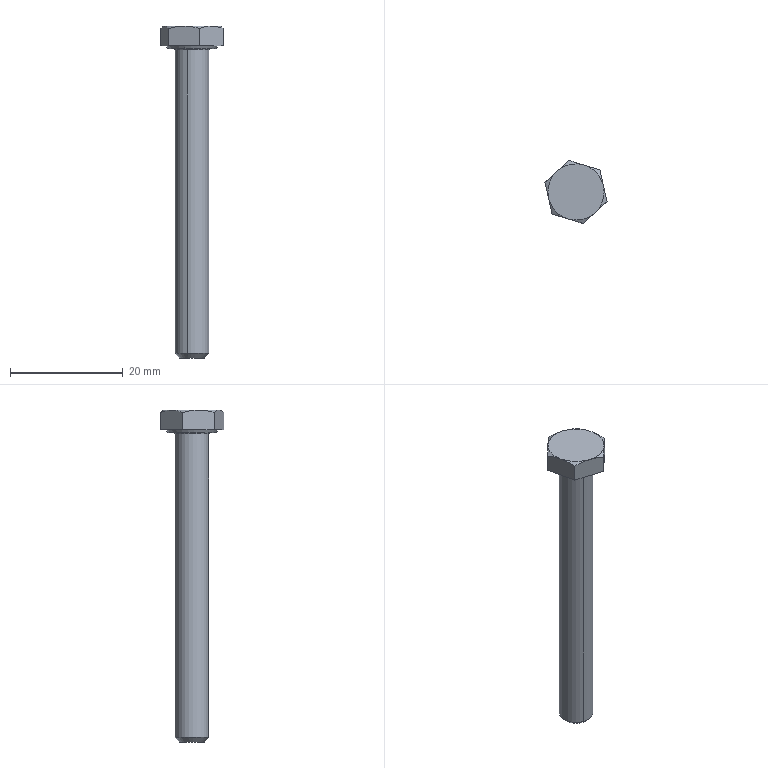Part | STEP file | BFACE2-18 | 1 solid | 24 faces | box 11.042 x 11.251 x 59 mm | volume 1883 mm3 | cone 10 | plane 10 | cylinder 2 | torus 2 | commonest cylinder face diameters 6 x2
STEP:
#1=CARTESIAN_POINT('',(-616.616,-367.304,3117.75));
#2=VERTEX_POINT('',#1);
#3=CARTESIAN_POINT('',(-614.861,-361.566,3117.75));
#4=VERTEX_POINT('',#3);
#5=CARTESIAN_POINT('',(-615.738,-364.435,3117.75));
#6=DIRECTION('',(0.,0.,1.));
#7=DIRECTION('',(-0.2924,-0.9563,0.));
#8=AXIS2_PLACEMENT_3D('',#5,#6,#7);
#9=CIRCLE('',#8,3.);
#10=EDGE_CURVE('',#2,#4,#9,.T.);
#11=ORIENTED_EDGE('',*,*,#10,.F.);
#12=CARTESIAN_POINT('',(-616.616,-367.304,3063.8));
#13=VERTEX_POINT('',#12);
#14=CARTESIAN_POINT('',(-616.616,-367.304,3122.));
#15=DIRECTION('',(0.,0.,1.));
#16=VECTOR('',#15,1000.);
#17=LINE('',#14,#16);
#18=EDGE_CURVE('',#13,#2,#17,.T.);
#19=ORIENTED_EDGE('',*,*,#18,.F.);
#20=CARTESIAN_POINT('',(-614.861,-361.566,3063.8));
#21=VERTEX_POINT('',#20);
#22=CARTESIAN_POINT('',(-615.738,-364.435,3063.8));
#23=DIRECTION('',(0.,0.,1.));
#24=DIRECTION('',(0.2924,0.9563,0.));
#25=AXIS2_PLACEMENT_3D('',#22,#23,#24);
#26=CIRCLE('',#25,3.);
#27=EDGE_CURVE('',#13,#21,#26,.T.);
#28=ORIENTED_EDGE('',*,*,#27,.T.);
#29=CARTESIAN_POINT('',(-614.861,-361.566,3122.));
#30=DIRECTION('',(0.,0.,1.));
#31=VECTOR('',#30,1000.);
#32=LINE('',#29,#31);
#33=EDGE_CURVE('',#21,#4,#32,.T.);
#34=ORIENTED_EDGE('',*,*,#33,.T.);
#35=EDGE_LOOP('',(#11,#19,#28,#34));
#36=FACE_OUTER_BOUND('',#35,.T.);
#37=CARTESIAN_POINT('',(-615.738,-364.435,3122.));
#38=DIRECTION('',(0.,0.,-1.));
#39=DIRECTION('',(-0.2924,-0.9563,0.));
#40=AXIS2_PLACEMENT_3D('',#37,#38,#39);
#41=CYLINDRICAL_SURFACE('',#40,3.);
#42=ADVANCED_FACE('',(#36),#41,.T.);
#43=CARTESIAN_POINT('',(-615.095,-362.331,3063.));
#44=VERTEX_POINT('',#43);
#45=CARTESIAN_POINT('',(-616.382,-366.539,3063.));
#46=VERTEX_POINT('',#45);
#47=CARTESIAN_POINT('',(-615.738,-364.435,3063.));
#48=DIRECTION('',(0.,0.,-1.));
#49=DIRECTION('',(0.2924,0.9563,0.));
#50=AXIS2_PLACEMENT_3D('',#47,#48,#49);
#51=CIRCLE('',#50,2.2);
#52=EDGE_CURVE('',#44,#46,#51,.T.);
#53=ORIENTED_EDGE('',*,*,#52,.F.);
#54=CARTESIAN_POINT('',(-615.095,-362.331,3063.));
#55=DIRECTION('',(0.2068,0.6762,0.7071));
#56=VECTOR('',#55,1000.);
#57=LINE('',#54,#56);
#58=EDGE_CURVE('',#44,#21,#57,.T.);
#59=ORIENTED_EDGE('',*,*,#58,.T.);
#60=ORIENTED_EDGE('',*,*,#27,.F.);
#61=CARTESIAN_POINT('',(-616.382,-366.539,3063.));
#62=DIRECTION('',(-0.2068,-0.6762,0.7071));
#63=VECTOR('',#62,1000.);
#64=LINE('',#61,#63);
#65=EDGE_CURVE('',#46,#13,#64,.T.);
#66=ORIENTED_EDGE('',*,*,#65,.F.);
#67=EDGE_LOOP('',(#53,#59,#60,#66));
#68=FACE_OUTER_BOUND('',#67,.T.);
#69=CARTESIAN_POINT('',(-615.738,-364.435,3063.));
#70=DIRECTION('',(0.,0.,1.));
#71=DIRECTION('',(0.2924,0.9563,0.));
#72=AXIS2_PLACEMENT_3D('',#69,#70,#71);
#73=CONICAL_SURFACE('',#72,2.2,0.7854);
#74=ADVANCED_FACE('',(#68),#73,.T.);
#75=CARTESIAN_POINT('',(-614.788,-361.327,3118.));
#76=VERTEX_POINT('',#75);
#77=CARTESIAN_POINT('',(-616.689,-367.543,3118.));
#78=VERTEX_POINT('',#77);
#79=CARTESIAN_POINT('',(-615.738,-364.435,3118.));
#80=DIRECTION('',(0.,0.,1.));
#81=DIRECTION('',(-0.2924,-0.9563,0.));
#82=AXIS2_PLACEMENT_3D('',#79,#80,#81);
#83=CIRCLE('',#82,3.25);
#84=EDGE_CURVE('',#76,#78,#83,.T.);
#85=ORIENTED_EDGE('',*,*,#84,.F.);
#86=CARTESIAN_POINT('',(-614.788,-361.327,3117.75));
#87=DIRECTION('',(0.9563,-0.2924,0.));
#88=DIRECTION('',(-0.2924,-0.9563,0.));
#89=AXIS2_PLACEMENT_3D('',#86,#87,#88);
#90=CIRCLE('',#89,0.25);
#91=EDGE_CURVE('',#76,#4,#90,.T.);
#92=ORIENTED_EDGE('',*,*,#91,.T.);
#93=CARTESIAN_POINT('',(-615.738,-364.435,3117.75));
#94=DIRECTION('',(0.,0.,1.));
#95=DIRECTION('',(-0.2924,-0.9563,0.));
#96=AXIS2_PLACEMENT_3D('',#93,#94,#95);
#97=CIRCLE('',#96,3.);
#98=EDGE_CURVE('',#4,#2,#97,.T.);
#99=ORIENTED_EDGE('',*,*,#98,.T.);
#100=CARTESIAN_POINT('',(-616.689,-367.543,3117.75));
#101=DIRECTION('',(-0.9563,0.2924,0.));
#102=DIRECTION('',(0.2924,0.9563,0.));
#103=AXIS2_PLACEMENT_3D('',#100,#101,#102);
#104=CIRCLE('',#103,0.25);
#105=EDGE_CURVE('',#78,#2,#104,.T.);
#106=ORIENTED_EDGE('',*,*,#105,.F.);
#107=EDGE_LOOP('',(#85,#92,#99,#106));
#108=FACE_OUTER_BOUND('',#107,.T.);
#109=CARTESIAN_POINT('',(-615.738,-364.435,3117.75));
#110=DIRECTION('',(0.,0.,1.));
#111=DIRECTION('',(0.2924,0.9563,0.));
#112=AXIS2_PLACEMENT_3D('',#109,#110,#111);
#113=TOROIDAL_SURFACE('',#112,3.25,0.25);
#114=ADVANCED_FACE('',(#108),#113,.F.);
#115=CARTESIAN_POINT('',(-616.999,-368.559,3118.));
#116=VERTEX_POINT('',#115);
#117=CARTESIAN_POINT('',(-614.477,-360.311,3118.));
#118=VERTEX_POINT('',#117);
#119=CARTESIAN_POINT('',(-615.738,-364.435,3118.));
#120=DIRECTION('',(0.,0.,1.));
#121=DIRECTION('',(-0.2924,-0.9563,0.));
#122=AXIS2_PLACEMENT_3D('',#119,#120,#121);
#123=CIRCLE('',#122,4.312);
#124=EDGE_CURVE('',#116,#118,#123,.T.);
#125=ORIENTED_EDGE('',*,*,#124,.T.);
#126=CARTESIAN_POINT('',(-614.393,-360.035,3118.5));
#127=VERTEX_POINT('',#126);
#128=CARTESIAN_POINT('',(-614.393,-360.035,3118.5));
#129=DIRECTION('',(0.1462,0.4781,0.866));
#130=VECTOR('',#129,1000.);
#131=LINE('',#128,#130);
#132=EDGE_CURVE('',#118,#127,#131,.T.);
#133=ORIENTED_EDGE('',*,*,#132,.T.);
#134=CARTESIAN_POINT('',(-617.084,-368.835,3118.5));
#135=VERTEX_POINT('',#134);
#136=CARTESIAN_POINT('',(-615.738,-364.435,3118.5));
#137=DIRECTION('',(0.,0.,1.));
#138=DIRECTION('',(-0.2924,-0.9563,0.));
#139=AXIS2_PLACEMENT_3D('',#136,#137,#138);
#140=CIRCLE('',#139,4.601);
#141=EDGE_CURVE('',#135,#127,#140,.T.);
#142=ORIENTED_EDGE('',*,*,#141,.F.);
#143=CARTESIAN_POINT('',(-617.084,-368.835,3118.5));
#144=DIRECTION('',(-0.1462,-0.4781,0.866));
#145=VECTOR('',#144,1000.);
#146=LINE('',#143,#145);
#147=EDGE_CURVE('',#116,#135,#146,.T.);
#148=ORIENTED_EDGE('',*,*,#147,.F.);
#149=EDGE_LOOP('',(#125,#133,#142,#148));
#150=FACE_OUTER_BOUND('',#149,.T.);
#151=CARTESIAN_POINT('',(-615.738,-364.435,3118.5));
#152=DIRECTION('',(0.,0.,1.));
#153=DIRECTION('',(0.2924,0.9563,0.));
#154=AXIS2_PLACEMENT_3D('',#151,#152,#153);
#155=CONICAL_SURFACE('',#154,4.601,0.5236);
#156=ADVANCED_FACE('',(#150),#155,.T.);
#157=ORIENTED_EDGE('',*,*,#124,.F.);
#158=CARTESIAN_POINT('',(-615.738,-364.435,3118.));
#159=DIRECTION('',(0.,0.,1.));
#160=DIRECTION('',(-0.2924,-0.9563,0.));
#161=AXIS2_PLACEMENT_3D('',#158,#159,#160);
#162=CIRCLE('',#161,4.312);
#163=EDGE_CURVE('',#118,#116,#162,.T.);
#164=ORIENTED_EDGE('',*,*,#163,.F.);
#165=EDGE_LOOP('',(#157,#164));
#166=FACE_OUTER_BOUND('',#165,.T.);
#167=CARTESIAN_POINT('',(-615.738,-364.435,3118.));
#168=DIRECTION('',(0.,0.,1.));
#169=DIRECTION('',(-0.2924,-0.9563,0.));
#170=AXIS2_PLACEMENT_3D('',#167,#168,#169);
#171=CIRCLE('',#170,3.25);
#172=EDGE_CURVE('',#78,#76,#171,.T.);
#173=ORIENTED_EDGE('',*,*,#172,.T.);
#174=ORIENTED_EDGE('',*,*,#84,.T.);
#175=EDGE_LOOP('',(#173,#174));
#176=FACE_BOUND('',#175,.T.);
#177=CARTESIAN_POINT('',(-610.217,-366.123,3118.));
#178=DIRECTION('',(0.,0.,-1.));
#179=DIRECTION('',(-0.2924,-0.9563,0.));
#180=AXIS2_PLACEMENT_3D('',#177,#178,#179);
#181=PLANE('',#180);
#182=ADVANCED_FACE('',(#166,#176),#181,.T.);
#183=CARTESIAN_POINT('',(-611.516,-360.498,3118.5));
#184=VERTEX_POINT('',#183);
#185=CARTESIAN_POINT('',(-610.217,-366.123,3118.5));
#186=VERTEX_POINT('',#185);
#187=CARTESIAN_POINT('',(-611.516,-360.498,3118.5));
#188=DIRECTION('',(0.2249,-0.9744,0.));
#189=VECTOR('',#188,1000.);
#190=LINE('',#187,#189);
#191=EDGE_CURVE('',#184,#186,#190,.T.);
#192=ORIENTED_EDGE('',*,*,#191,.F.);
#193=CARTESIAN_POINT('',(-611.516,-360.498,3121.553));
#194=VERTEX_POINT('',#193);
#195=CARTESIAN_POINT('',(-611.516,-360.498,3118.));
#196=DIRECTION('',(0.,0.,1.));
#197=VECTOR('',#196,1000.);
#198=LINE('',#195,#197);
#199=EDGE_CURVE('',#184,#194,#198,.T.);
#200=ORIENTED_EDGE('',*,*,#199,.T.);
#201=CARTESIAN_POINT('',(-610.866,-363.311,3122.));
#202=VERTEX_POINT('',#201);
#203=CARTESIAN_POINT('',(-610.866,-363.311,3122.));
#204=CARTESIAN_POINT('',(-611.088,-362.351,3122.));
#205=CARTESIAN_POINT('',(-611.303,-361.417,3121.826));
#206=CARTESIAN_POINT('',(-611.516,-360.498,3121.553));
#207=B_SPLINE_CURVE_WITH_KNOTS('',3,(#203,#204,#205,#206),.UNSPECIFIED.,.F.,.F.,(4,4),(0.,0.002921),.UNSPECIFIED.);
#208=EDGE_CURVE('',#202,#194,#207,.T.);
#209=ORIENTED_EDGE('',*,*,#208,.F.);
#210=CARTESIAN_POINT('',(-610.217,-366.123,3121.553));
#211=VERTEX_POINT('',#210);
#212=CARTESIAN_POINT('',(-610.217,-366.123,3121.553));
#213=CARTESIAN_POINT('',(-610.429,-365.204,3121.826));
#214=CARTESIAN_POINT('',(-610.645,-364.271,3122.));
#215=CARTESIAN_POINT('',(-610.866,-363.311,3122.));
#216=B_SPLINE_CURVE_WITH_KNOTS('',3,(#212,#213,#214,#215),.UNSPECIFIED.,.F.,.F.,(4,4),(0.,0.002921),.UNSPECIFIED.);
#217=EDGE_CURVE('',#211,#202,#216,.T.);
#218=ORIENTED_EDGE('',*,*,#217,.F.);
#219=CARTESIAN_POINT('',(-610.217,-366.123,3118.));
#220=DIRECTION('',(0.,0.,1.));
#221=VECTOR('',#220,1000.);
#222=LINE('',#219,#221);
#223=EDGE_CURVE('',#186,#211,#222,.T.);
#224=ORIENTED_EDGE('',*,*,#223,.F.);
#225=EDGE_LOOP('',(#192,#200,#209,#218,#224));
#226=FACE_OUTER_BOUND('',#225,.T.);
#227=CARTESIAN_POINT('',(-611.516,-360.498,3118.));
#228=DIRECTION('',(-0.9744,-0.2249,0.));
#229=DIRECTION('',(0.2249,-0.9744,0.));
#230=AXIS2_PLACEMENT_3D('',#227,#228,#229);
#231=PLANE('',#230);
#232=ADVANCED_FACE('',(#226),#231,.F.);
#233=CARTESIAN_POINT('',(-614.44,-370.061,3118.5));
#234=VERTEX_POINT('',#233);
#235=CARTESIAN_POINT('',(-610.217,-366.123,3118.5));
#236=DIRECTION('',(-0.7314,-0.682,0.));
#237=VECTOR('',#236,1000.);
#238=LINE('',#235,#237);
#239=EDGE_CURVE('',#186,#234,#238,.T.);
#240=ORIENTED_EDGE('',*,*,#239,.F.);
#241=ORIENTED_EDGE('',*,*,#223,.T.);
#242=CARTESIAN_POINT('',(-612.329,-368.092,3122.));
#243=VERTEX_POINT('',#242);
#244=CARTESIAN_POINT('',(-612.329,-368.092,3122.));
#245=CARTESIAN_POINT('',(-611.608,-367.42,3122.));
#246=CARTESIAN_POINT('',(-610.907,-366.767,3121.826));
#247=CARTESIAN_POINT('',(-610.217,-366.123,3121.553));
#248=B_SPLINE_CURVE_WITH_KNOTS('',3,(#244,#245,#246,#247),.UNSPECIFIED.,.F.,.F.,(4,4),(0.,0.002921),.UNSPECIFIED.);
#249=EDGE_CURVE('',#243,#211,#248,.T.);
#250=ORIENTED_EDGE('',*,*,#249,.F.);
#251=CARTESIAN_POINT('',(-614.44,-370.061,3121.553));
#252=VERTEX_POINT('',#251);
#253=CARTESIAN_POINT('',(-614.44,-370.061,3121.553));
#254=CARTESIAN_POINT('',(-613.75,-369.418,3121.826));
#255=CARTESIAN_POINT('',(-613.049,-368.764,3122.));
#256=CARTESIAN_POINT('',(-612.329,-368.092,3122.));
#257=B_SPLINE_CURVE_WITH_KNOTS('',3,(#253,#254,#255,#256),.UNSPECIFIED.,.F.,.F.,(4,4),(0.,0.002921),.UNSPECIFIED.);
#258=EDGE_CURVE('',#252,#243,#257,.T.);
#259=ORIENTED_EDGE('',*,*,#258,.F.);
#260=CARTESIAN_POINT('',(-614.44,-370.061,3118.));
#261=DIRECTION('',(0.,0.,1.));
#262=VECTOR('',#261,1000.);
#263=LINE('',#260,#262);
#264=EDGE_CURVE('',#234,#252,#263,.T.);
#265=ORIENTED_EDGE('',*,*,#264,.F.);
#266=EDGE_LOOP('',(#240,#241,#250,#259,#265));
#267=FACE_OUTER_BOUND('',#266,.T.);
#268=CARTESIAN_POINT('',(-610.217,-366.123,3118.));
#269=DIRECTION('',(-0.682,0.7314,0.));
#270=DIRECTION('',(-0.7314,-0.682,0.));
#271=AXIS2_PLACEMENT_3D('',#268,#269,#270);
#272=PLANE('',#271);
#273=ADVANCED_FACE('',(#267),#272,.F.);
#274=CARTESIAN_POINT('',(-619.961,-368.372,3118.5));
#275=VERTEX_POINT('',#274);
#276=CARTESIAN_POINT('',(-614.44,-370.061,3118.5));
#277=DIRECTION('',(-0.9563,0.2924,0.));
#278=VECTOR('',#277,1000.);
#279=LINE('',#276,#278);
#280=EDGE_CURVE('',#234,#275,#279,.T.);
#281=ORIENTED_EDGE('',*,*,#280,.F.);
#282=ORIENTED_EDGE('',*,*,#264,.T.);
#283=CARTESIAN_POINT('',(-617.2,-369.217,3122.));
#284=VERTEX_POINT('',#283);
#285=CARTESIAN_POINT('',(-617.2,-369.217,3122.));
#286=CARTESIAN_POINT('',(-616.258,-369.505,3122.));
#287=CARTESIAN_POINT('',(-615.342,-369.785,3121.826));
#288=CARTESIAN_POINT('',(-614.44,-370.061,3121.553));
#289=B_SPLINE_CURVE_WITH_KNOTS('',3,(#285,#286,#287,#288),.UNSPECIFIED.,.F.,.F.,(4,4),(0.,0.002921),.UNSPECIFIED.);
#290=EDGE_CURVE('',#284,#252,#289,.T.);
#291=ORIENTED_EDGE('',*,*,#290,.F.);
#292=CARTESIAN_POINT('',(-619.961,-368.372,3121.553));
#293=VERTEX_POINT('',#292);
#294=CARTESIAN_POINT('',(-619.961,-368.372,3121.553));
#295=CARTESIAN_POINT('',(-619.059,-368.648,3121.826));
#296=CARTESIAN_POINT('',(-618.143,-368.928,3122.));
#297=CARTESIAN_POINT('',(-617.2,-369.217,3122.));
#298=B_SPLINE_CURVE_WITH_KNOTS('',3,(#294,#295,#296,#297),.UNSPECIFIED.,.F.,.F.,(4,4),(0.,0.002921),.UNSPECIFIED.);
#299=EDGE_CURVE('',#293,#284,#298,.T.);
#300=ORIENTED_EDGE('',*,*,#299,.F.);
#301=CARTESIAN_POINT('',(-619.961,-368.372,3118.));
#302=DIRECTION('',(0.,0.,1.));
#303=VECTOR('',#302,1000.);
#304=LINE('',#301,#303);
#305=EDGE_CURVE('',#275,#293,#304,.T.);
#306=ORIENTED_EDGE('',*,*,#305,.F.);
#307=EDGE_LOOP('',(#281,#282,#291,#300,#306));
#308=FACE_OUTER_BOUND('',#307,.T.);
#309=CARTESIAN_POINT('',(-614.44,-370.061,3118.));
#310=DIRECTION('',(0.2924,0.9563,0.));
#311=DIRECTION('',(0.,0.,-1.));
#312=AXIS2_PLACEMENT_3D('',#309,#310,#311);
#313=PLANE('',#312);
#314=ADVANCED_FACE('',(#308),#313,.F.);
#315=CARTESIAN_POINT('',(-621.259,-362.747,3118.5));
#316=VERTEX_POINT('',#315);
#317=CARTESIAN_POINT('',(-621.259,-362.747,3118.5));
#318=DIRECTION('',(-0.2249,0.9744,0.));
#319=VECTOR('',#318,1000.);
#320=LINE('',#317,#319);
#321=EDGE_CURVE('',#275,#316,#320,.T.);
#322=ORIENTED_EDGE('',*,*,#321,.F.);
#323=ORIENTED_EDGE('',*,*,#305,.T.);
#324=CARTESIAN_POINT('',(-620.61,-365.56,3122.));
#325=VERTEX_POINT('',#324);
#326=CARTESIAN_POINT('',(-620.61,-365.56,3122.));
#327=CARTESIAN_POINT('',(-620.389,-366.52,3122.));
#328=CARTESIAN_POINT('',(-620.173,-367.453,3121.826));
#329=CARTESIAN_POINT('',(-619.961,-368.372,3121.553));
#330=B_SPLINE_CURVE_WITH_KNOTS('',3,(#326,#327,#328,#329),.UNSPECIFIED.,.F.,.F.,(4,4),(0.,0.002921),.UNSPECIFIED.);
#331=EDGE_CURVE('',#325,#293,#330,.T.);
#332=ORIENTED_EDGE('',*,*,#331,.F.);
#333=CARTESIAN_POINT('',(-621.259,-362.747,3121.553));
#334=VERTEX_POINT('',#333);
#335=CARTESIAN_POINT('',(-621.259,-362.747,3121.553));
#336=CARTESIAN_POINT('',(-621.047,-363.666,3121.826));
#337=CARTESIAN_POINT('',(-620.832,-364.6,3122.));
#338=CARTESIAN_POINT('',(-620.61,-365.56,3122.));
#339=B_SPLINE_CURVE_WITH_KNOTS('',3,(#335,#336,#337,#338),.UNSPECIFIED.,.F.,.F.,(4,4),(0.,0.002921),.UNSPECIFIED.);
#340=EDGE_CURVE('',#334,#325,#339,.T.);
#341=ORIENTED_EDGE('',*,*,#340,.F.);
#342=CARTESIAN_POINT('',(-621.259,-362.747,3118.));
#343=DIRECTION('',(0.,0.,1.));
#344=VECTOR('',#343,1000.);
#345=LINE('',#342,#344);
#346=EDGE_CURVE('',#316,#334,#345,.T.);
#347=ORIENTED_EDGE('',*,*,#346,.F.);
#348=EDGE_LOOP('',(#322,#323,#332,#341,#347));
#349=FACE_OUTER_BOUND('',#348,.T.);
#350=CARTESIAN_POINT('',(-621.259,-362.747,3118.));
#351=DIRECTION('',(0.9744,0.2249,0.));
#352=DIRECTION('',(-0.2249,0.9744,0.));
#353=AXIS2_PLACEMENT_3D('',#350,#351,#352);
#354=PLANE('',#353);
#355=ADVANCED_FACE('',(#349),#354,.F.);
#356=CARTESIAN_POINT('',(-617.037,-358.81,3118.5));
#357=VERTEX_POINT('',#356);
#358=CARTESIAN_POINT('',(-617.037,-358.81,3118.5));
#359=DIRECTION('',(0.7314,0.682,0.));
#360=VECTOR('',#359,1000.);
#361=LINE('',#358,#360);
#362=EDGE_CURVE('',#316,#357,#361,.T.);
#363=ORIENTED_EDGE('',*,*,#362,.F.);
#364=ORIENTED_EDGE('',*,*,#346,.T.);
#365=CARTESIAN_POINT('',(-619.148,-360.778,3122.));
#366=VERTEX_POINT('',#365);
#367=CARTESIAN_POINT('',(-619.148,-360.778,3122.));
#368=CARTESIAN_POINT('',(-619.869,-361.45,3122.));
#369=CARTESIAN_POINT('',(-620.57,-362.104,3121.826));
#370=CARTESIAN_POINT('',(-621.259,-362.747,3121.553));
#371=B_SPLINE_CURVE_WITH_KNOTS('',3,(#367,#368,#369,#370),.UNSPECIFIED.,.F.,.F.,(4,4),(0.,0.002921),.UNSPECIFIED.);
#372=EDGE_CURVE('',#366,#334,#371,.T.);
#373=ORIENTED_EDGE('',*,*,#372,.F.);
#374=CARTESIAN_POINT('',(-617.037,-358.81,3121.553));
#375=VERTEX_POINT('',#374);
#376=CARTESIAN_POINT('',(-617.037,-358.81,3121.553));
#377=CARTESIAN_POINT('',(-617.726,-359.453,3121.826));
#378=CARTESIAN_POINT('',(-618.427,-360.106,3122.));
#379=CARTESIAN_POINT('',(-619.148,-360.778,3122.));
#380=B_SPLINE_CURVE_WITH_KNOTS('',3,(#376,#377,#378,#379),.UNSPECIFIED.,.F.,.F.,(4,4),(0.,0.002921),.UNSPECIFIED.);
#381=EDGE_CURVE('',#375,#366,#380,.T.);
#382=ORIENTED_EDGE('',*,*,#381,.F.);
#383=CARTESIAN_POINT('',(-617.037,-358.81,3118.));
#384=DIRECTION('',(0.,0.,1.));
#385=VECTOR('',#384,1000.);
#386=LINE('',#383,#385);
#387=EDGE_CURVE('',#357,#375,#386,.T.);
#388=ORIENTED_EDGE('',*,*,#387,.F.);
#389=EDGE_LOOP('',(#363,#364,#373,#382,#388));
#390=FACE_OUTER_BOUND('',#389,.T.);
#391=CARTESIAN_POINT('',(-617.037,-358.81,3118.));
#392=DIRECTION('',(0.682,-0.7314,0.));
#393=DIRECTION('',(0.7314,0.682,0.));
#394=AXIS2_PLACEMENT_3D('',#391,#392,#393);
#395=PLANE('',#394);
#396=ADVANCED_FACE('',(#390),#395,.F.);
#397=CARTESIAN_POINT('',(-611.516,-360.498,3118.5));
#398=DIRECTION('',(0.9563,-0.2924,0.));
#399=VECTOR('',#398,1000.);
#400=LINE('',#397,#399);
#401=EDGE_CURVE('',#357,#184,#400,.T.);
#402=ORIENTED_EDGE('',*,*,#401,.F.);
#403=ORIENTED_EDGE('',*,*,#387,.T.);
#404=CARTESIAN_POINT('',(-614.276,-359.654,3122.));
#405=VERTEX_POINT('',#404);
#406=CARTESIAN_POINT('',(-614.276,-359.654,3122.));
#407=CARTESIAN_POINT('',(-615.218,-359.366,3122.));
#408=CARTESIAN_POINT('',(-616.135,-359.085,3121.826));
#409=CARTESIAN_POINT('',(-617.037,-358.81,3121.553));
#410=B_SPLINE_CURVE_WITH_KNOTS('',3,(#406,#407,#408,#409),.UNSPECIFIED.,.F.,.F.,(4,4),(0.,0.002921),.UNSPECIFIED.);
#411=EDGE_CURVE('',#405,#375,#410,.T.);
#412=ORIENTED_EDGE('',*,*,#411,.F.);
#413=CARTESIAN_POINT('',(-611.516,-360.498,3121.553));
#414=CARTESIAN_POINT('',(-612.417,-360.222,3121.826));
#415=CARTESIAN_POINT('',(-613.334,-359.942,3122.));
#416=CARTESIAN_POINT('',(-614.276,-359.654,3122.));
#417=B_SPLINE_CURVE_WITH_KNOTS('',3,(#413,#414,#415,#416),.UNSPECIFIED.,.F.,.F.,(4,4),(0.,0.002921),.UNSPECIFIED.);
#418=EDGE_CURVE('',#194,#405,#417,.T.);
#419=ORIENTED_EDGE('',*,*,#418,.F.);
#420=ORIENTED_EDGE('',*,*,#199,.F.);
#421=EDGE_LOOP('',(#402,#403,#412,#419,#420));
#422=FACE_OUTER_BOUND('',#421,.T.);
#423=CARTESIAN_POINT('',(-611.516,-360.498,3118.));
#424=DIRECTION('',(-0.2924,-0.9563,0.));
#425=DIRECTION('',(0.9563,-0.2924,0.));
#426=AXIS2_PLACEMENT_3D('',#423,#424,#425);
#427=PLANE('',#426);
#428=ADVANCED_FACE('',(#422),#427,.F.);
#429=ORIENTED_EDGE('',*,*,#381,.T.);
#430=CARTESIAN_POINT('',(-615.738,-364.435,3122.));
#431=DIRECTION('',(0.,0.,-1.));
#432=DIRECTION('',(0.2924,0.9563,0.));
#433=AXIS2_PLACEMENT_3D('',#430,#431,#432);
#434=CIRCLE('',#433,5.);
#435=EDGE_CURVE('',#366,#405,#434,.T.);
#436=ORIENTED_EDGE('',*,*,#435,.T.);
#437=ORIENTED_EDGE('',*,*,#411,.T.);
#438=EDGE_LOOP('',(#429,#436,#437));
#439=FACE_OUTER_BOUND('',#438,.T.);
#440=CARTESIAN_POINT('',(-615.738,-364.435,3122.));
#441=DIRECTION('',(0.,0.,-1.));
#442=DIRECTION('',(-0.2924,-0.9563,0.));
#443=AXIS2_PLACEMENT_3D('',#440,#441,#442);
#444=CONICAL_SURFACE('',#443,5.,1.047);
#445=ADVANCED_FACE('',(#439),#444,.T.);
#446=ORIENTED_EDGE('',*,*,#340,.T.);
#447=CARTESIAN_POINT('',(-615.738,-364.435,3122.));
#448=DIRECTION('',(0.,0.,-1.));
#449=DIRECTION('',(0.2924,0.9563,0.));
#450=AXIS2_PLACEMENT_3D('',#447,#448,#449);
#451=CIRCLE('',#450,5.);
#452=EDGE_CURVE('',#325,#366,#451,.T.);
#453=ORIENTED_EDGE('',*,*,#452,.T.);
#454=ORIENTED_EDGE('',*,*,#372,.T.);
#455=EDGE_LOOP('',(#446,#453,#454));
#456=FACE_OUTER_BOUND('',#455,.T.);
#457=CARTESIAN_POINT('',(-615.738,-364.435,3122.));
#458=DIRECTION('',(0.,0.,-1.));
#459=DIRECTION('',(-0.2924,-0.9563,0.));
#460=AXIS2_PLACEMENT_3D('',#457,#458,#459);
#461=CONICAL_SURFACE('',#460,5.,1.047);
#462=ADVANCED_FACE('',(#456),#461,.T.);
#463=ORIENTED_EDGE('',*,*,#299,.T.);
#464=CARTESIAN_POINT('',(-615.738,-364.435,3122.));
#465=DIRECTION('',(0.,0.,-1.));
#466=DIRECTION('',(0.2924,0.9563,0.));
#467=AXIS2_PLACEMENT_3D('',#464,#465,#466);
#468=CIRCLE('',#467,5.);
#469=EDGE_CURVE('',#284,#325,#468,.T.);
#470=ORIENTED_EDGE('',*,*,#469,.T.);
#471=ORIENTED_EDGE('',*,*,#331,.T.);
#472=EDGE_LOOP('',(#463,#470,#471));
#473=FACE_OUTER_BOUND('',#472,.T.);
#474=CARTESIAN_POINT('',(-615.738,-364.435,3122.));
#475=DIRECTION('',(0.,0.,-1.));
#476=DIRECTION('',(-0.2924,-0.9563,0.));
#477=AXIS2_PLACEMENT_3D('',#474,#475,#476);
#478=CONICAL_SURFACE('',#477,5.,1.047);
#479=ADVANCED_FACE('',(#473),#478,.T.);
#480=ORIENTED_EDGE('',*,*,#290,.T.);
#481=ORIENTED_EDGE('',*,*,#258,.T.);
#482=CARTESIAN_POINT('',(-615.738,-364.435,3122.));
#483=DIRECTION('',(0.,0.,1.));
#484=DIRECTION('',(-0.2924,-0.9563,0.));
#485=AXIS2_PLACEMENT_3D('',#482,#483,#484);
#486=CIRCLE('',#485,5.);
#487=EDGE_CURVE('',#284,#243,#486,.T.);
#488=ORIENTED_EDGE('',*,*,#487,.F.);
#489=EDGE_LOOP('',(#480,#481,#488));
#490=FACE_OUTER_BOUND('',#489,.T.);
#491=CARTESIAN_POINT('',(-615.738,-364.435,3122.));
#492=DIRECTION('',(0.,0.,-1.));
#493=DIRECTION('',(-0.2924,-0.9563,0.));
#494=AXIS2_PLACEMENT_3D('',#491,#492,#493);
#495=CONICAL_SURFACE('',#494,5.,1.047);
#496=ADVANCED_FACE('',(#490),#495,.T.);
#497=ORIENTED_EDGE('',*,*,#249,.T.);
#498=ORIENTED_EDGE('',*,*,#217,.T.);
#499=CARTESIAN_POINT('',(-615.738,-364.435,3122.));
#500=DIRECTION('',(0.,0.,-1.));
#501=DIRECTION('',(0.2924,0.9563,0.));
#502=AXIS2_PLACEMENT_3D('',#499,#500,#501);
#503=CIRCLE('',#502,5.);
#504=EDGE_CURVE('',#202,#243,#503,.T.);
#505=ORIENTED_EDGE('',*,*,#504,.T.);
#506=EDGE_LOOP('',(#497,#498,#505));
#507=FACE_OUTER_BOUND('',#506,.T.);
#508=CARTESIAN_POINT('',(-615.738,-364.435,3122.));
#509=DIRECTION('',(0.,0.,-1.));
#510=DIRECTION('',(-0.2924,-0.9563,0.));
#511=AXIS2_PLACEMENT_3D('',#508,#509,#510);
#512=CONICAL_SURFACE('',#511,5.,1.047);
#513=ADVANCED_FACE('',(#507),#512,.T.);
#514=ORIENTED_EDGE('',*,*,#208,.T.);
#515=ORIENTED_EDGE('',*,*,#418,.T.);
#516=CARTESIAN_POINT('',(-615.738,-364.435,3122.));
#517=DIRECTION('',(0.,0.,-1.));
#518=DIRECTION('',(0.2924,0.9563,0.));
#519=AXIS2_PLACEMENT_3D('',#516,#517,#518);
#520=CIRCLE('',#519,5.);
#521=EDGE_CURVE('',#405,#202,#520,.T.);
#522=ORIENTED_EDGE('',*,*,#521,.T.);
#523=EDGE_LOOP('',(#514,#515,#522));
#524=FACE_OUTER_BOUND('',#523,.T.);
#525=CARTESIAN_POINT('',(-615.738,-364.435,3122.));
#526=DIRECTION('',(0.,0.,-1.));
#527=DIRECTION('',(-0.2924,-0.9563,0.));
#528=AXIS2_PLACEMENT_3D('',#525,#526,#527);
#529=CONICAL_SURFACE('',#528,5.,1.047);
#530=ADVANCED_FACE('',(#524),#529,.T.);
#531=ORIENTED_EDGE('',*,*,#521,.F.);
#532=ORIENTED_EDGE('',*,*,#435,.F.);
#533=ORIENTED_EDGE('',*,*,#452,.F.);
#534=ORIENTED_EDGE('',*,*,#469,.F.);
#535=ORIENTED_EDGE('',*,*,#487,.T.);
#536=ORIENTED_EDGE('',*,*,#504,.F.);
#537=EDGE_LOOP('',(#531,#532,#533,#534,#535,#536));
#538=FACE_OUTER_BOUND('',#537,.T.);
#539=CARTESIAN_POINT('',(-610.217,-366.123,3122.));
#540=DIRECTION('',(0.,0.,-1.));
#541=DIRECTION('',(-0.2924,-0.9563,0.));
#542=AXIS2_PLACEMENT_3D('',#539,#540,#541);
#543=PLANE('',#542);
#544=ADVANCED_FACE('',(#538),#543,.F.);
#545=ORIENTED_EDGE('',*,*,#141,.T.);
#546=CARTESIAN_POINT('',(-615.738,-364.435,3118.5));
#547=DIRECTION('',(0.,0.,1.));
#548=DIRECTION('',(-0.2924,-0.9563,0.));
#549=AXIS2_PLACEMENT_3D('',#546,#547,#548);
#550=CIRCLE('',#549,4.601);
#551=EDGE_CURVE('',#127,#135,#550,.T.);
#552=ORIENTED_EDGE('',*,*,#551,.T.);
#553=EDGE_LOOP('',(#545,#552));
#554=FACE_BOUND('',#553,.T.);
#555=ORIENTED_EDGE('',*,*,#191,.T.);
#556=ORIENTED_EDGE('',*,*,#239,.T.);
#557=ORIENTED_EDGE('',*,*,#280,.T.);
#558=ORIENTED_EDGE('',*,*,#321,.T.);
#559=ORIENTED_EDGE('',*,*,#362,.T.);
#560=ORIENTED_EDGE('',*,*,#401,.T.);
#561=EDGE_LOOP('',(#555,#556,#557,#558,#559,#560));
#562=FACE_OUTER_BOUND('',#561,.T.);
#563=CARTESIAN_POINT('',(-611.338,-365.781,3118.5));
#564=DIRECTION('',(0.,0.,-1.));
#565=DIRECTION('',(-0.2924,-0.9563,0.));
#566=AXIS2_PLACEMENT_3D('',#563,#564,#565);
#567=PLANE('',#566);
#568=ADVANCED_FACE('',(#554,#562),#567,.T.);
#569=ORIENTED_EDGE('',*,*,#132,.F.);
#570=ORIENTED_EDGE('',*,*,#163,.T.);
#571=ORIENTED_EDGE('',*,*,#147,.T.);
#572=ORIENTED_EDGE('',*,*,#551,.F.);
#573=EDGE_LOOP('',(#569,#570,#571,#572));
#574=FACE_OUTER_BOUND('',#573,.T.);
#575=CARTESIAN_POINT('',(-615.738,-364.435,3118.5));
#576=DIRECTION('',(0.,0.,1.));
#577=DIRECTION('',(0.2924,0.9563,0.));
#578=AXIS2_PLACEMENT_3D('',#575,#576,#577);
#579=CONICAL_SURFACE('',#578,4.601,0.5236);
#580=ADVANCED_FACE('',(#574),#579,.T.);
#581=ORIENTED_EDGE('',*,*,#91,.F.);
#582=ORIENTED_EDGE('',*,*,#172,.F.);
#583=ORIENTED_EDGE('',*,*,#105,.T.);
#584=ORIENTED_EDGE('',*,*,#10,.T.);
#585=EDGE_LOOP('',(#581,#582,#583,#584));
#586=FACE_OUTER_BOUND('',#585,.T.);
#587=CARTESIAN_POINT('',(-615.738,-364.435,3117.75));
#588=DIRECTION('',(0.,0.,1.));
#589=DIRECTION('',(0.2924,0.9563,0.));
#590=AXIS2_PLACEMENT_3D('',#587,#588,#589);
#591=TOROIDAL_SURFACE('',#590,3.25,0.25);
#592=ADVANCED_FACE('',(#586),#591,.F.);
#593=CARTESIAN_POINT('',(-615.738,-364.435,3063.));
#594=DIRECTION('',(0.,0.,-1.));
#595=DIRECTION('',(0.2924,0.9563,0.));
#596=AXIS2_PLACEMENT_3D('',#593,#594,#595);
#597=CIRCLE('',#596,2.2);
#598=EDGE_CURVE('',#46,#44,#597,.T.);
#599=ORIENTED_EDGE('',*,*,#598,.T.);
#600=ORIENTED_EDGE('',*,*,#52,.T.);
#601=EDGE_LOOP('',(#599,#600));
#602=FACE_OUTER_BOUND('',#601,.T.);
#603=CARTESIAN_POINT('',(-615.738,-364.435,3063.));
#604=DIRECTION('',(0.,0.,-1.));
#605=DIRECTION('',(-0.2924,-0.9563,0.));
#606=AXIS2_PLACEMENT_3D('',#603,#604,#605);
#607=PLANE('',#606);
#608=ADVANCED_FACE('',(#602),#607,.T.);
#609=ORIENTED_EDGE('',*,*,#58,.F.);
#610=ORIENTED_EDGE('',*,*,#598,.F.);
#611=ORIENTED_EDGE('',*,*,#65,.T.);
#612=CARTESIAN_POINT('',(-615.738,-364.435,3063.8));
#613=DIRECTION('',(0.,0.,1.));
#614=DIRECTION('',(0.2924,0.9563,0.));
#615=AXIS2_PLACEMENT_3D('',#612,#613,#614);
#616=CIRCLE('',#615,3.);
#617=EDGE_CURVE('',#21,#13,#616,.T.);
#618=ORIENTED_EDGE('',*,*,#617,.F.);
#619=EDGE_LOOP('',(#609,#610,#611,#618));
#620=FACE_OUTER_BOUND('',#619,.T.);
#621=CARTESIAN_POINT('',(-615.738,-364.435,3063.));
#622=DIRECTION('',(0.,0.,1.));
#623=DIRECTION('',(0.2924,0.9563,0.));
#624=AXIS2_PLACEMENT_3D('',#621,#622,#623);
#625=CONICAL_SURFACE('',#624,2.2,0.7854);
#626=ADVANCED_FACE('',(#620),#625,.T.);
#627=ORIENTED_EDGE('',*,*,#18,.T.);
#628=ORIENTED_EDGE('',*,*,#98,.F.);
#629=ORIENTED_EDGE('',*,*,#33,.F.);
#630=ORIENTED_EDGE('',*,*,#617,.T.);
#631=EDGE_LOOP('',(#627,#628,#629,#630));
#632=FACE_OUTER_BOUND('',#631,.T.);
#633=CARTESIAN_POINT('',(-615.738,-364.435,3122.));
#634=DIRECTION('',(0.,0.,-1.));
#635=DIRECTION('',(-0.2924,-0.9563,0.));
#636=AXIS2_PLACEMENT_3D('',#633,#634,#635);
#637=CYLINDRICAL_SURFACE('',#636,3.);
#638=ADVANCED_FACE('',(#632),#637,.T.);
#639=CLOSED_SHELL('',(#42,#74,#114,#156,#182,#232,#273,#314,#355,#396,#428,#445,#462,#479,#496,#513,#530,#544,#568,#580,#592,#608,#626,#638));
#640=MANIFOLD_SOLID_BREP('',#639);
#641=CARTESIAN_POINT('',(0.,0.,0.));
#642=DIRECTION('',(0.,0.,1.));
#643=DIRECTION('',(1.,0.,0.));
#644=AXIS2_PLACEMENT_3D('',#641,#642,#643);
#645=(LENGTH_UNIT()NAMED_UNIT(*)SI_UNIT(.MILLI.,.METRE.));
#646=UNCERTAINTY_MEASURE_WITH_UNIT(LENGTH_MEASURE(0.00001),#645,'','');
#647=(NAMED_UNIT(*)PLANE_ANGLE_UNIT()SI_UNIT($,.RADIAN.));
#648=(NAMED_UNIT(*)SI_UNIT($,.STERADIAN.)SOLID_ANGLE_UNIT());
#649=(GEOMETRIC_REPRESENTATION_CONTEXT(3)GLOBAL_UNCERTAINTY_ASSIGNED_CONTEXT((#646))GLOBAL_UNIT_ASSIGNED_CONTEXT((#645,#647,#648))REPRESENTATION_CONTEXT('',''));
#650=ADVANCED_BREP_SHAPE_REPRESENTATION('',(#640,#644),#649);